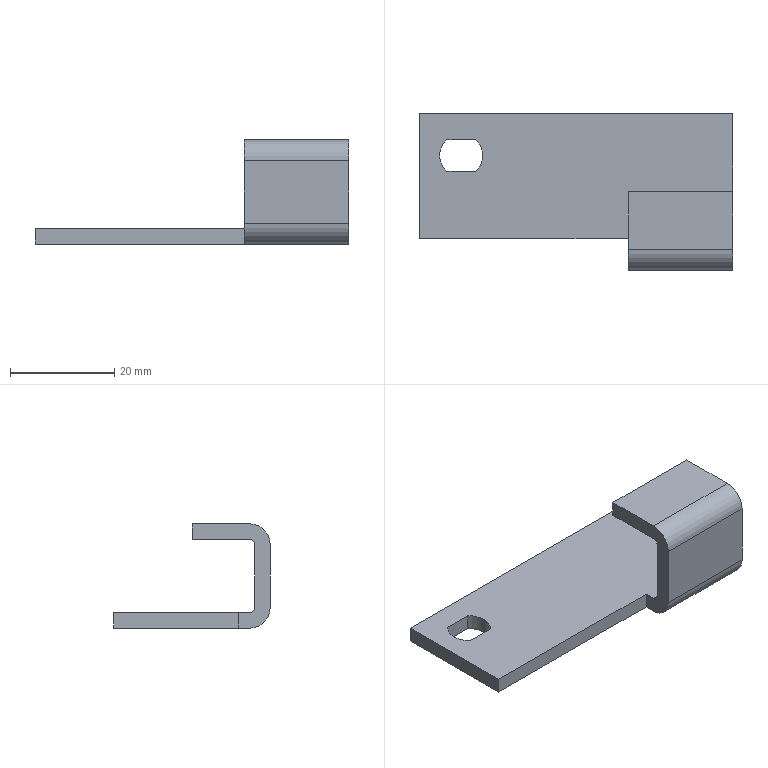Part | STEP file | 8xs161054 | 1 solid | 21 faces | box 60 x 30 x 20 mm | volume 6156 mm3 | plane 14 | cylinder 7 | commonest cylinder face diameters 8.2 x3 2 x2 8 x2